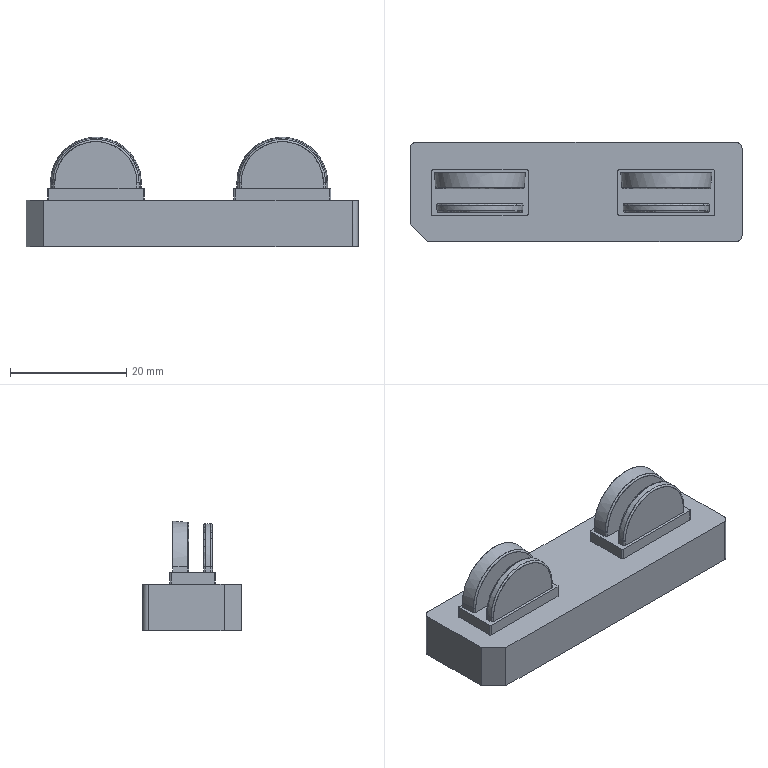NC program | PowerMill | posted by the shop | part box 57 x 17 x 18.807 mm
Lines 5595 to 7074 of 381081:
( TOOL ID   D4C_1_1 )
( TOOL DIA. 4. TIP RAD 0 LENGTH 66. )
( Z = -10.94 )
T2 M6
T28
G91 G28 Z0
G0 G90 G54
M08
S18000 M3
X0 Y0 M8
G43 Z9.797 H2
X-18.031 Y6.252
Z.788
G1 Z-.412 F3600
X-18.041 Y6.232 F6000
G3 X-17.952 Y5.967 I.177 J-.089
G1 X-16.594 Y5.288
X-14.886
X-14.398 Y5.259
X-13.942 Y5.125
X-13.421 Y4.791
X-13.258 Y4.637
X-12.93 Y4.148
X-12.77 Y3.66
X-12.737 Y3.172
X-12.828 Y2.684
X-12.975 Y2.196
X-13.19 Y1.708
X-13.925 Y.244
X-14.275 Y-.244
X-14.398 Y-.373
X-14.886 Y-.748
X-15.374 Y-1.024
X-15.862 Y-1.159
X-16.239 Y-1.22
X-16.747
X-17.326 Y-1.124
X-17.814 Y-.934
X-18.144 Y-.732
X-18.79 Y-.186
X-19.067 Y.244
X-19.81 Y1.708
X-20.026 Y2.196
X-20.172 Y2.684
X-20.26 Y3.172
X-20.23 Y3.66
X-20.07 Y4.148
X-19.766 Y4.607
X-19.278 Y5.011
X-19.057 Y5.125
X-18.79 Y5.218
X-18.302 Y5.288
X-16.594
X-18.019 Y6.246 Z-.612
X-18.029 Y6.226
G3 X-17.94 Y5.961 I.177 J-.089
G1 X-16.594 Y5.288
X-14.886
X-14.857 Y5.286
X-14.851
X-13.91
X-13.421 Y5.206
X-13.192 Y5.125
X-12.933 Y4.988
X-12.506 Y4.637
X-12.178 Y4.148
X-12.018 Y3.66
X-11.986 Y3.172
X-12.07 Y2.684
X-12.632 Y.732
X-12.74 Y.244
X-12.933 Y-.196
X-13.395 Y-.732
X-13.91 Y-1.072
X-14.072 Y-1.136
G3 X-14.179 Y-1.409 I.073 J-.186
G1 X-14.033 Y-1.708
X-13.947 Y-2.196
X-13.978 Y-2.684
X-14.121 Y-3.172
X-14.456 Y-3.66
X-15.374 Y-4.401
X-15.862 Y-4.645
X-16.35 Y-4.744
X-16.838 Y-4.721
X-17.145 Y-4.637
X-17.326 Y-4.571
X-17.814 Y-4.255
X-18.302 Y-3.885
X-18.545 Y-3.66
X-18.79 Y-3.324
X-18.869 Y-3.172
X-19.031 Y-2.684
X-19.054 Y-2.196
X-18.961 Y-1.708
X-18.814 Y-1.398
G3 X-18.911 Y-1.131 I-.181 J.086
G1 X-19.278 Y-.963
X-19.6 Y-.732
X-19.766 Y-.584
X-20.034 Y-.244
X-20.261 Y.244
X-20.368 Y.732
X-20.929 Y2.684
X-21.013 Y3.172
X-20.981 Y3.66
X-20.822 Y4.148
X-20.742 Y4.294
X-20.493 Y4.637
X-20.254 Y4.856
X-19.808 Y5.125
X-19.278 Y5.27
X-18.79 Y5.288
X-18.035
X-16.594
X-18.033 Y6.253 Z-.811
X-18.043 Y6.234
G3 X-17.955 Y5.968 I.177 J-.089
G1 X-16.594 Y5.288
X-14.886
X-14.866 Y5.287
X-13.421 Y5.286
X-12.933 Y5.205
X-12.706 Y5.125
X-12.445 Y4.987
X-12.019 Y4.637
X-11.691 Y4.148
X-11.53 Y3.66
X-11.5 Y3.172
X-12.119 Y.244
X-12.34 Y-.244
X-12.445 Y-.396
X-12.752 Y-.732
X-13.033 Y-.937
G3 X-13.075 Y-1.22 I.119 J-.162
G1 X-12.854 Y-1.708
X-12.762 Y-2.196
X-12.792 Y-2.684
X-13.017 Y-3.66
X-13.199 Y-4.148
X-13.421 Y-4.495
X-13.552 Y-4.637
X-13.91 Y-4.927
X-14.234 Y-5.125
X-14.398 Y-5.2
X-14.886 Y-5.341
X-15.374 Y-5.435
X-16.838 Y-5.478
X-17.814 Y-5.411
X-18.302 Y-5.294
X-18.765 Y-5.125
X-19.278 Y-4.789
X-19.449 Y-4.637
X-19.766 Y-4.216
X-19.976 Y-3.66
X-20.208 Y-2.684
X-20.238 Y-2.196
X-20.146 Y-1.708
X-19.925 Y-1.22
G3 X-19.968 Y-.955 I-.168 J.108
G1 X-20.248 Y-.732
X-20.658 Y-.244
X-20.742 Y-.098
X-20.882 Y.244
X-21.5 Y3.172
X-21.467 Y3.66
X-21.309 Y4.148
X-21.23 Y4.295
X-20.981 Y4.637
X-20.742 Y4.858
X-20.296 Y5.125
X-19.766 Y5.27
X-19.282 Y5.288
X-18.797
X-18.793
X-18.79
X-18.089
X-18.009
X-16.594
X-18.032 Y6.253 Z-1.01
X-18.042 Y6.233
G3 X-17.953 Y5.968 I.177 J-.089
G1 X-16.594 Y5.288
X-13.421
X-12.933 Y5.283
X-12.445 Y5.19
X-12.266 Y5.125
X-11.957 Y4.956
X-11.581 Y4.637
X-11.469 Y4.5
X-11.252 Y4.148
X-11.093 Y3.66
X-11.062 Y3.172
X-11.3 Y1.708
X-11.603 Y.244
X-11.825 Y-.244
X-12.216 Y-.732
X-12.392 Y-.87
G3 X-12.445 Y-1.123 I.123 J-.158
G1 X-12.177 Y-1.708
X-12.082 Y-2.196
X-12.114 Y-2.684
X-12.276 Y-3.66
X-12.445 Y-4.14
X-12.801 Y-4.637
X-12.933 Y-4.774
X-13.416 Y-5.125
X-13.91 Y-5.323
X-14.398 Y-5.437
X-14.886 Y-5.499
X-17.326 Y-5.524
X-18.302 Y-5.484
X-18.79 Y-5.404
X-19.278 Y-5.253
X-19.581 Y-5.125
X-19.766 Y-5.018
X-20.197 Y-4.637
X-20.55 Y-4.148
X-20.725 Y-3.66
X-20.889 Y-2.684
X-20.918 Y-2.196
X-20.826 Y-1.708
X-20.614 Y-1.22
X-20.57 Y-1.156
X-20.536 Y-1.086
G3 X-20.615 Y-.863 I-.194 J.057
G1 X-20.782 Y-.732
X-21.174 Y-.244
X-21.397 Y.244
X-21.718 Y1.798
X-21.939 Y3.172
X-21.907 Y3.66
X-21.747 Y4.148
X-21.419 Y4.637
X-21.23 Y4.816
X-20.742 Y5.12
X-20.254 Y5.263
X-19.766 Y5.288
X-16.594
X-18.033 Y6.253 Z-1.209
X-18.042 Y6.234
G3 X-17.954 Y5.968 I.177 J-.089
G1 X-16.594 Y5.288
X-12.933
X-12.445 Y5.273
X-11.957 Y5.15
X-11.469 Y4.875
X-11.208 Y4.637
X-10.981 Y4.333
X-10.879 Y4.148
X-10.72 Y3.66
X-10.689 Y3.172
X-11.168 Y.244
X-11.389 Y-.244
X-11.773 Y-.732
X-11.898 Y-.834
G3 X-11.938 Y-1.1 I.126 J-.155
G1 X-11.858 Y-1.22
X-11.656 Y-1.708
X-11.561 Y-2.196
X-11.591 Y-2.684
X-11.685 Y-3.172
X-11.742 Y-3.66
X-11.917 Y-4.148
X-12.247 Y-4.637
X-12.445 Y-4.839
X-12.86 Y-5.125
X-13.421 Y-5.364
X-13.91 Y-5.474
X-14.398 Y-5.513
X-16.945 Y-5.52
X-17.326 Y-5.524
X-17.39 Y-5.521
X-17.394
X-18.302 Y-5.524
X-18.79 Y-5.504
X-19.278 Y-5.435
X-19.766 Y-5.3
X-20.254 Y-5.06
X-20.752 Y-4.637
X-21.083 Y-4.148
X-21.23 Y-3.769
X-21.315 Y-3.172
X-21.409 Y-2.684
X-21.439 Y-2.196
X-21.347 Y-1.708
X-21.23 Y-1.389
X-21.144 Y-1.22
X-21.063 Y-1.101
G3 X-21.103 Y-.834 I-.166 J.112
G1 X-21.23 Y-.731
X-21.611 Y-.244
X-21.718 Y-.05
X-21.834 Y.244
X-22.311 Y3.172
X-22.28 Y3.66
X-22.12 Y4.148
X-21.792 Y4.637
X-21.23 Y5.066
X-20.742 Y5.241
X-20.254 Y5.288
X-16.594
X-18.029 Y6.251 Z-1.408
X-18.039 Y6.232
G3 X-17.95 Y5.966 I.177 J-.089
G1 X-16.594 Y5.288
X-12.933
X-12.929
X-12.445
X-11.957 Y5.25
X-11.551 Y5.125
X-10.981 Y4.755
X-10.866 Y4.637
X-10.537 Y4.148
X-10.377 Y3.66
X-10.346 Y3.172
X-10.406 Y2.684
X-10.792 Y.244
X-10.981 Y-.187
X-11.388 Y-.732
X-11.494 Y-.818
G3 X-11.532 Y-1.086 I.127 J-.155
G1 X-11.441 Y-1.22
X-11.234 Y-1.708
X-11.144 Y-2.196
X-11.172 Y-2.684
X-11.298 Y-3.66
X-11.473 Y-4.148
X-11.799 Y-4.637
X-11.957 Y-4.803
X-12.401 Y-5.125
X-12.933 Y-5.364
X-13.421 Y-5.481
X-13.91 Y-5.518
X-14.398 Y-5.524
X-18.79
X-19.278 Y-5.508
X-19.766 Y-5.445
X-20.254 Y-5.299
X-20.742 Y-5.037
X-21.201 Y-4.637
X-21.527 Y-4.148
X-21.7 Y-3.66
X-21.828 Y-2.684
X-21.857 Y-2.196
X-21.766 Y-1.708
X-21.557 Y-1.22
X-21.462 Y-1.081
G3 X-21.476 Y-.841 I-.159 J.111
G1 X-21.495 Y-.819
X-21.718 Y-.62
X-21.988 Y-.244
X-22.208 Y.244
X-22.526 Y2.196
X-22.654 Y3.172
X-22.624 Y3.66
X-22.463 Y4.148
X-22.206 Y4.554
X-21.718 Y4.985
X-21.45 Y5.125
X-21.23 Y5.204
X-20.742 Y5.286
X-20.271
X-20.254 Y5.288
X-16.594
X-18.031 Y6.253 Z-1.608
X-18.041 Y6.233
G3 X-17.953 Y5.967 I.177 J-.089
G1 X-16.594 Y5.288
X-12.933
X-12.929
X-12.445
X-12.416 Y5.286
X-12.409
X-11.957 Y5.285
X-11.469 Y5.201
X-11.255 Y5.125
X-10.981 Y4.978
X-10.57 Y4.637
X-10.242 Y4.148
X-10.082 Y3.66
X-10.051 Y3.172
X-10.387 Y.732
X-10.475 Y.244
X-10.691 Y-.244
X-10.981 Y-.648
X-11.15 Y-.797
G3 X-11.182 Y-1.061 I.132 J-.15
G1 X-11.071 Y-1.22
X-10.981 Y-1.4
X-10.872 Y-1.708
X-10.781 Y-2.196
X-10.811 Y-2.684
X-10.925 Y-3.66
X-10.981 Y-3.867
X-11.1 Y-4.148
X-11.406 Y-4.637
X-11.988 Y-5.125
X-12.445 Y-5.34
X-12.933 Y-5.469
X-13.421 Y-5.518
X-13.91 Y-5.524
X-19.278
X-19.766 Y-5.505
X-20.254 Y-5.427
X-20.742 Y-5.269
X-21.011 Y-5.125
X-21.23 Y-4.972
X-21.594 Y-4.637
X-21.718 Y-4.47
X-21.901 Y-4.148
X-22.076 Y-3.66
X-22.206 Y-2.559
X-22.219 Y-2.196
X-22.128 Y-1.708
X-21.929 Y-1.22
X-21.821 Y-1.066
G3 X-21.857 Y-.798 I-.164 J.114
G1 X-21.936 Y-.732
X-22.206 Y-.41
X-22.309 Y-.244
X-22.525 Y.244
X-22.613 Y.732
X-22.949 Y3.172
X-22.918 Y3.66
X-22.758 Y4.148
X-22.43 Y4.637
X-22.206 Y4.845
X-21.744 Y5.125
X-21.23 Y5.268
X-20.742 Y5.288
X-20.155
X-16.594
X-18.032 Y6.253 Z-1.807
X-18.042 Y6.234
G3 X-17.954 Y5.968 I.177 J-.089
G1 X-16.594 Y5.288
X-11.957
X-11.469 Y5.265
X-10.979 Y5.125
X-10.493 Y4.826
X-10.294 Y4.637
X-10.005 Y4.225
X-9.806 Y3.66
X-9.774 Y3.172
X-10.034 Y1.22
X-10.174 Y.244
X-10.381 Y-.244
X-10.493 Y-.425
X-10.753 Y-.732
X-10.809 Y-.778
X-10.857 Y-.832
G3 X-10.853 Y-1.055 I.168 J-.108
G1 X-10.738 Y-1.22
X-10.539 Y-1.708
X-10.45 Y-2.196
X-10.48 Y-2.684
X-10.587 Y-3.66
X-10.76 Y-4.148
X-11.073 Y-4.637
X-11.469 Y-4.994
X-11.653 Y-5.125
X-11.957 Y-5.283
X-12.445 Y-5.444
X-12.933 Y-5.513
X-13.421 Y-5.524
X-19.766
X-20.254 Y-5.494
X-20.742 Y-5.389
X-21.23 Y-5.192
X-21.718 Y-4.848
X-21.926 Y-4.637
X-22.206 Y-4.21
X-22.414 Y-3.66
X-22.488 Y-2.929
X-22.549 Y-2.196
X-22.461 Y-1.708
X-22.262 Y-1.22
X-22.146 Y-1.055
G3 X-22.192 Y-.778 I-.165 J.115
G1 X-22.247 Y-.732
X-22.62 Y-.244
X-22.826 Y.244
X-22.909 Y.732
X-23.226 Y3.172
X-23.195 Y3.66
X-23.035 Y4.148
X-22.706 Y4.637
X-22.206 Y5.033
X-22.021 Y5.125
X-21.718 Y5.226
X-21.23 Y5.288
X-16.594
X-18.029 Y6.251 Z-2.006
X-18.039 Y6.232
G3 X-17.95 Y5.966 I.177 J-.089
G1 X-16.594 Y5.288
X-11.957
X-11.946 Y5.287
X-11.469
X-10.981 Y5.215
X-10.724 Y5.125
X-10.493 Y5.006
X-10.039 Y4.637
X-9.711 Y4.148
X-9.551 Y3.66
X-9.52 Y3.172
X-9.815 Y.732
X-9.906 Y.244
X-10.121 Y-.244
X-10.493 Y-.731
X-10.562 Y-.793
X-10.606 Y-.874
X-10.61 Y-.963
X-10.574 Y-1.044
X-10.493 Y-1.155
X-10.257 Y-1.708
X-10.172 Y-2.196
X-10.301 Y-3.66
X-10.47 Y-4.148
X-10.773 Y-4.637
X-10.981 Y-4.847
X-11.337 Y-5.125
X-11.469 Y-5.201
X-11.957 Y-5.401
X-12.445 Y-5.497
X-12.933 Y-5.524
X-13.417
X-13.419
X-13.421
X-19.766
X-19.786 Y-5.523
X-20.254
X-20.742 Y-5.474
X-21.23 Y-5.334
X-21.662 Y-5.125
X-22.206 Y-4.659
X-22.53 Y-4.148
X-22.699 Y-3.66
X-22.828 Y-2.196
X-22.694 Y-1.55
X-22.545 Y-1.22
X-22.421 Y-1.044
G3 X-22.439 Y-.791 I-.163 J.115
G1 X-22.694 Y-.523
X-22.879 Y-.244
X-23.094 Y.244
X-23.183 Y.711
X-23.48 Y3.172
X-23.449 Y3.66
X-23.289 Y4.148
X-23.183 Y4.343
X-22.961 Y4.637
X-22.694 Y4.879
X-22.274 Y5.125
X-21.718 Y5.273
X-21.23 Y5.288
X-20.394
X-16.594
X-18.029 Y6.251 Z-2.205
X-18.038 Y6.232
G3 X-17.95 Y5.966 I.177 J-.089
G1 X-16.594 Y5.288
X-11.469
X-10.981 Y5.262
X-10.503 Y5.125
X-10.005 Y4.815
X-9.818 Y4.637
X-9.517 Y4.202
X-9.33 Y3.66
X-9.299 Y3.172
X-9.575 Y.732
X-9.659 Y.244
X-9.863 Y-.244
X-10.005 Y-.468
X-10.235 Y-.732
X-10.299 Y-.791
X-10.34 Y-.868
X-10.344 Y-.955
X-10.311 Y-1.036
X-10.181 Y-1.22
X-10.005 Y-1.632
X-9.898 Y-2.196
X-9.919 Y-2.684
X-10.005 Y-3.554
X-10.196 Y-4.148
X-10.499 Y-4.637
X-11.063 Y-5.125
X-11.469 Y-5.323
X-11.957 Y-5.47
X-12.445 Y-5.523
X-12.915
X-12.933 Y-5.524
X-13.417
X-13.419
X-13.421
X-19.766
X-19.769
X-19.771
X-20.257
X-20.742 Y-5.509
X-21.23 Y-5.428
X-21.718 Y-5.246
X-21.936 Y-5.125
X-22.206 Y-4.92
X-22.501 Y-4.637
X-22.694 Y-4.363
X-22.804 Y-4.148
X-22.975 Y-3.66
X-23.036 Y-3.172
X-23.102 Y-2.196
X-23.017 Y-1.708
X-22.819 Y-1.22
X-22.689 Y-1.037
G3 X-22.721 Y-.77 I-.163 J.115
G1 X-22.765 Y-.732
X-23.138 Y-.244
X-23.341 Y.244
X-23.425 Y.732
X-23.7 Y3.172
X-23.671 Y3.655
X-23.51 Y4.148
X-23.182 Y4.637
X-22.694 Y5.025
X-22.495 Y5.125
X-22.206 Y5.224
X-21.718 Y5.288
X-16.594
X-18.033 Y6.253 Z-2.405
X-18.043 Y6.234
G3 X-17.954 Y5.968 I.177 J-.089
G1 X-16.594 Y5.288
X-11.469
X-11.421 Y5.285
X-11.416
X-10.981
X-10.493 Y5.2
X-10.282 Y5.125
X-10.005 Y4.976
X-9.597 Y4.637
X-9.269 Y4.148
X-9.109 Y3.66
X-9.078 Y3.172
X-9.353 Y.732
X-9.437 Y.244
X-9.645 Y-.244
X-10.018 Y-.732
X-10.092 Y-.813
X-10.12 Y-.92
X-10.109 Y-.977
X-10.083 Y-1.029
X-9.947 Y-1.22
X-9.75 Y-1.708
X-9.662 Y-2.196
X-9.781 Y-3.66
X-9.951 Y-4.148
X-10.254 Y-4.637
X-10.493 Y-4.877
X-10.807 Y-5.125
X-10.981 Y-5.224
X-11.469 Y-5.421
X-11.957 Y-5.506
X-12.445 Y-5.524
X-20.742
X-21.23 Y-5.485
X-21.718 Y-5.356
X-22.194 Y-5.125
X-22.694 Y-4.694
X-23.049 Y-4.148
X-23.219 Y-3.66
X-23.337 Y-2.196
X-23.25 Y-1.708
X-23.183 Y-1.499
X-23.053 Y-1.22
X-22.912 Y-1.021
G3 X-22.932 Y-.765 I-.163 J.116
G1 X-23.183 Y-.509
X-23.355 Y-.244
X-23.563 Y.244
X-23.647 Y.732
X-23.921 Y3.172
X-23.891 Y3.66
X-23.73 Y4.148
X-23.403 Y4.637
X-23.183 Y4.843
X-22.716 Y5.125
X-22.206 Y5.268
X-21.723 Y5.288
X-21.238
X-16.594
X-18.021 Y6.247 Z-2.604
X-18.031 Y6.228
G3 X-17.942 Y5.962 I.177 J-.089
G1 X-16.594 Y5.288
X-11.507
X-10.981
X-10.493 Y5.251
X-10.085 Y5.125
X-9.517 Y4.754
X-9.4 Y4.637
X-9.072 Y4.148
X-8.912 Y3.66
X-8.88 Y3.172
X-9.138 Y.732
X-9.226 Y.244
X-9.428 Y-.244
X-9.517 Y-.392
X-9.801 Y-.732
X-9.871 Y-.812
X-9.896 Y-.915
X-9.886 Y-.972
X-9.859 Y-1.023
X-9.719 Y-1.22
X-9.522 Y-1.708
X-9.438 Y-2.196
X-9.468 Y-2.684
X-9.557 Y-3.66
X-9.723 Y-4.148
X-10.005 Y-4.609
X-10.579 Y-5.125
X-10.981 Y-5.325
X-11.469 Y-5.474
X-11.957 Y-5.524
X-20.742
X-21.23 Y-5.514
X-21.718 Y-5.432
X-22.206 Y-5.243
X-22.422 Y-5.125
X-22.694 Y-4.914
X-22.973 Y-4.637
X-23.183 Y-4.335
X-23.276 Y-4.148
X-23.443 Y-3.66
X-23.561 Y-2.196
X-23.478 Y-1.708
X-23.281 Y-1.22
X-23.141 Y-1.023
G3 X-23.179 Y-.75 I-.164 J.116
G1 X-23.199 Y-.732
X-23.573 Y-.244
X-23.774 Y.244
X-23.862 Y.732
X-24.12 Y3.172
X-24.088 Y3.66
X-23.928 Y4.148
X-23.6 Y4.637
X-23.183 Y4.984
X-22.915 Y5.125
X-22.694 Y5.203
X-22.206 Y5.286
X-21.775
X-21.718 Y5.288
X-21.238
X-16.594
X-18.03 Y6.252 Z-2.803
X-18.04 Y6.232
G3 X-17.951 Y5.967 I.177 J-.089
G1 X-16.594 Y5.288
X-10.981
X-10.493 Y5.277
X-10.005 Y5.164
X-9.517 Y4.902
X-9.221 Y4.637
X-9.029 Y4.391
X-8.892 Y4.148
X-8.732 Y3.66
X-8.701 Y3.172
X-8.951 Y.732
X-9.035 Y.244
X-9.237 Y-.244
X-9.517 Y-.636
X-9.638 Y-.756
G3 X-9.662 Y-1.012 I.141 J-.142
G1 X-9.517 Y-1.22
X-9.32 Y-1.708
X-9.232 Y-2.196
X-9.252 Y-2.684
X-9.346 Y-3.66
X-9.512 Y-4.148
X-9.816 Y-4.637
X-10.005 Y-4.836
X-10.358 Y-5.125
X-10.493 Y-5.203
X-10.981 Y-5.411
X-11.469 Y-5.504
X-11.957 Y-5.524
X-21.23
X-21.718 Y-5.48
X-22.206 Y-5.342
X-22.64 Y-5.125
X-23.184 Y-4.637
X-23.488 Y-4.148
X-23.654 Y-3.66
X-23.712 Y-3.172
X-23.768 Y-2.196
X-23.68 Y-1.708
X-23.483 Y-1.22
X-23.34 Y-1.015
G3 X-23.347 Y-.779 I-.158 J.113
G1 X-23.365 Y-.757
X-23.39 Y-.732
X-23.671 Y-.396
X-23.763 Y-.244
X-23.965 Y.244
X-24.049 Y.732
X-24.299 Y3.172
X-24.268 Y3.66
X-24.108 Y4.148
X-23.78 Y4.637
X-23.671 Y4.747
X-23.183 Y5.083
X-22.694 Y5.249
X-22.206 Y5.288
X-21.713
X-16.594
X-18.027 Y6.251 Z-3.003
X-18.037 Y6.231
G3 X-17.949 Y5.965 I.177 J-.089
G1 X-16.594 Y5.288
X-10.981
X-10.97
X-10.493
X-10.005 Y5.221
X-9.726 Y5.125
X-9.517 Y5.019
X-9.042 Y4.637
X-8.712 Y4.148
X-8.553 Y3.66
X-8.521 Y3.172
X-8.768 Y.732
X-8.851 Y.244
X-9.029 Y-.195
X-9.428 Y-.732
G3 X-9.473 Y-1.01 I.123 J-.163
G1 X-9.326 Y-1.22
X-9.129 Y-1.708
X-9.043 Y-2.196
X-9.153 Y-3.66
X-9.322 Y-4.148
X-9.517 Y-4.495
X-9.626 Y-4.637
X-10.005 Y-5.008
X-10.168 Y-5.125
X-10.493 Y-5.295
X-10.981 Y-5.461
X-11.469 Y-5.523
X-11.933
X-11.937
X-11.957 Y-5.524
X-20.738
X-21.228
X-21.718 Y-5.508
X-22.206 Y-5.413
X-22.694 Y-5.204
X-22.831 Y-5.125
X-23.183 Y-4.839
X-23.374 Y-4.637
X-23.671 Y-4.165
X-23.847 Y-3.66
X-23.957 Y-2.196
X-23.871 Y-1.708
X-23.671 Y-1.215
X-23.526 Y-1.009
G3 X-23.548 Y-.752 I-.164 J.115
G1 X-23.671 Y-.63
X-23.945 Y-.244
X-24.149 Y.244
X-24.233 Y.732
X-24.479 Y3.172
X-24.447 Y3.66
X-24.288 Y4.148
X-24.159 Y4.376
X-23.959 Y4.637
X-23.671 Y4.895
X-23.274 Y5.125
X-22.694 Y5.275
X-22.206 Y5.288
X-20.301
X-16.594
X-18.032 Y6.253 Z-3.202
X-18.041 Y6.233
G3 X-17.953 Y5.967 I.177 J-.089
G1 X-16.594 Y5.288
X-12.922
X-10.493
X-10.005 Y5.257
X-9.56 Y5.125
X-9.029 Y4.788
X-8.875 Y4.637
X-8.546 Y4.148
X-8.387 Y3.66
X-8.355 Y3.172
X-8.603 Y.732
X-8.687 Y.244
X-8.882 Y-.244
X-9.029 Y-.473
X-9.28 Y-.749
G3 X-9.298 Y-.997 I.148 J-.135
G1 X-9.145 Y-1.22
X-9.029 Y-1.461
X-8.948 Y-1.708
X-8.87 Y-2.196
X-8.976 Y-3.66
X-9.134 Y-4.148
X-9.437 Y-4.637
X-9.978 Y-5.125
X-10.493 Y-5.376
X-10.981 Y-5.492
X-11.469 Y-5.524
X-13.289
X-20.738
X-21.23
X-21.252 Y-5.523
X-21.718
X-22.206 Y-5.462
X-22.694 Y-5.296
X-23.022 Y-5.125
X-23.183 Y-5.01
X-23.563 Y-4.637
X-23.671 Y-4.496
X-23.866 Y-4.148
X-24.024 Y-3.66
X-24.131 Y-2.196
X-24.052 Y-1.708
X-23.855 Y-1.22
X-23.707 Y-1.004
G3 X-23.741 Y-.739 I-.166 J.113
G1 X-23.748 Y-.732
X-24.117 Y-.244
X-24.313 Y.244
X-24.397 Y.732
X-24.645 Y3.172
X-24.613 Y3.66
X-24.454 Y4.148
X-24.159 Y4.598
X-23.671 Y5.007
X-23.438 Y5.125
X-23.183 Y5.215
X-22.694 Y5.287
X-22.22
X-22.206 Y5.288
X-20.301
X-16.594
X-18.032 Y6.253 Z-3.401
X-18.042 Y6.234
G3 X-17.954 Y5.968 I.177 J-.089
G1 X-16.594 Y5.288
X-10.493
X-10.005 Y5.276
X-9.517 Y5.163
X-9.029 Y4.899
X-8.735 Y4.637
X-8.541 Y4.387
X-8.406 Y4.148
X-8.247 Y3.66
X-8.215 Y3.172
X-8.447 Y.732
X-8.533 Y.244
X-8.73 Y-.244
X-9.029 Y-.657
X-9.093 Y-.719
X-9.147 Y-.789
G3 X-9.135 Y-.999 I.176 J-.095
G1 X-9.029 Y-1.149
X-8.789 Y-1.708
X-8.703 Y-2.196
X-8.721 Y-2.684
X-8.813 Y-3.66
X-8.975 Y-4.148
X-9.278 Y-4.637
X-9.517 Y-4.892
X-9.814 Y-5.125
X-10.005 Y-5.231
X-10.493 Y-5.432
X-10.981 Y-5.515
X-11.469 Y-5.524
X-21.718
X-22.206 Y-5.491
X-22.694 Y-5.371
X-23.183 Y-5.127
X-23.671 Y-4.693
X-24.025 Y-4.148
X-24.159 Y-3.771
X-24.243 Y-3.172
X-24.296 Y-2.196
X-24.211 Y-1.708
X-24.014 Y-1.22
X-23.858 Y-.993
G3 X-23.882 Y-.737 I-.166 J.113
G1 X-24.159 Y-.426
X-24.271 Y-.244
X-24.468 Y.244
X-24.553 Y.732
X-24.785 Y3.172
X-24.753 Y3.66
X-24.593 Y4.148
X-24.265 Y4.637
X-24.159 Y4.743
X-23.671 Y5.082
X-23.183 Y5.248
X-22.694 Y5.288
X-16.594
X-18.022 Y6.248 Z-3.6
X-18.032 Y6.228
G3 X-17.943 Y5.963 I.177 J-.089
G1 X-16.594 Y5.288
X-10.493
X-10.451 Y5.287
X-10.449
X-10.005
X-9.517 Y5.211
X-9.275 Y5.125
X-9.029 Y4.997
X-8.589 Y4.637
X-8.261 Y4.148
X-8.101 Y3.66
X-8.07 Y3.172
X-8.297 Y.732
X-8.381 Y.244
X-8.541 Y-.176
X-8.946 Y-.732
G3 X-8.98 Y-.997 I.132 J-.152
G1 X-8.827 Y-1.22
X-8.63 Y-1.708
X-8.552 Y-2.196
X-8.659 Y-3.66
X-8.817 Y-4.148
X-9.029 Y-4.52
X-9.119 Y-4.637
X-9.517 Y-5.027
X-9.655 Y-5.125
X-10.005 Y-5.311
X-10.493 Y-5.469
X-10.981 Y-5.524
X-21.718
X-22.206 Y-5.513
X-22.694 Y-5.425
X-23.183 Y-5.217
X-23.345 Y-5.125
X-23.671 Y-4.864
X-23.88 Y-4.637
X-24.159 Y-4.203
X-24.342 Y-3.66
X-24.449 Y-2.196
X-24.37 Y-1.708
X-24.159 Y-1.198
X-24.019 Y-.995
G3 X-24.04 Y-.743 I-.165 J.113
G1 X-24.159 Y-.621
X-24.424 Y-.244
X-24.619 Y.244
X-24.702 Y.732
X-24.93 Y3.172
X-24.899 Y3.66
X-24.738 Y4.148
X-24.647 Y4.318
X-24.41 Y4.637
X-24.159 Y4.867
X-23.725 Y5.125
X-23.183 Y5.272
X-22.694 Y5.288
X-22.062
X-16.594
X-18.029 Y6.252 Z-3.799
X-18.039 Y6.232
G3 X-17.95 Y5.966 I.177 J-.089
G1 X-16.594 Y5.288
X-10.005
X-9.517 Y5.244
X-9.029 Y5.074
X-8.541 Y4.727
X-8.453 Y4.637
X-8.124 Y4.148
X-7.965 Y3.66
X-7.933 Y3.172
X-8.164 Y.732
X-8.247 Y.244
X-8.441 Y-.244
X-8.541 Y-.407
X-8.831 Y-.742
G3 X-8.846 Y-.985 I.151 J-.131
G1 X-8.687 Y-1.22
X-8.49 Y-1.708
X-8.412 Y-2.196
X-8.516 Y-3.66
X-8.671 Y-4.148
X-8.974 Y-4.637
X-9.504 Y-5.125
X-10.005 Y-5.377
X-10.493 Y-5.494
X-10.981 Y-5.524
X-11.739
X-21.718
X-21.779 Y-5.523
X-22.206
X-22.694 Y-5.462
X-23.183 Y-5.297
X-23.496 Y-5.125
X-23.671 Y-4.998
X-24.026 Y-4.637
X-24.159 Y-4.459
X-24.329 Y-4.148
X-24.485 Y-3.66
X-24.587 Y-2.196
X-24.51 Y-1.708
X-24.313 Y-1.22
X-24.161 Y-.994
G3 X-24.177 Y-.752 I-.162 J.111
G1 X-24.185 Y-.742
X-24.194 Y-.732
X-24.559 Y-.244
X-24.753 Y.244
X-24.836 Y.732
X-25.067 Y3.172
X-25.035 Y3.66
X-24.875 Y4.148
X-24.647 Y4.518
X-24.547 Y4.637
X-24.159 Y4.966
X-23.861 Y5.125
X-23.671 Y5.196
X-23.183 Y5.284
X-22.694 Y5.288
X-16.594
X-18.032 Y6.253 Z-3.999
X-18.042 Y6.233
G3 X-17.953 Y5.968 I.177 J-.089
G1 X-16.594 Y5.288
X-10.005
X-9.517 Y5.267
X-9.016 Y5.125
X-8.541 Y4.835
X-8.33 Y4.637
X-8.002 Y4.148
X-7.842 Y3.66
X-7.811 Y3.172
X-8.03 Y.732
X-8.116 Y.244
X-8.315 Y-.244
X-8.541 Y-.575
X-8.694 Y-.739
G3 X-8.715 Y-.986 I.146 J-.136
G1 X-8.541 Y-1.248
X-8.358 Y-1.708
X-8.281 Y-2.196
X-8.299 Y-2.684
X-8.384 Y-3.66
X-8.541 Y-4.151
X-8.843 Y-4.637
X-9.029 Y-4.845
X-9.373 Y-5.125
X-10.005 Y-5.42
X-10.493 Y-5.513
X-10.981 Y-5.524
X-22.206
X-22.694 Y-5.486
X-23.183 Y-5.355
X-23.627 Y-5.125
X-24.159 Y-4.634
X-24.461 Y-4.148
X-24.616 Y-3.66
X-24.647 Y-3.48
X-24.719 Y-2.196
X-24.641 Y-1.708
X-24.445 Y-1.22
X-24.29 Y-.992
X-24.257 Y-.902
X-24.271 Y-.808
X-24.291 Y-.767
X-24.321 Y-.732
X-24.647 Y-.311
X-24.884 Y.244
X-24.97 Y.732
X-25.189 Y3.172
X-25.157 Y3.66
X-24.998 Y4.148
X-24.669 Y4.637
X-24.159 Y5.038
X-23.983 Y5.125
X-23.671 Y5.23
X-23.183 Y5.288
X-16.594
X-18.027 Y6.25 Z-4.198
X-18.037 Y6.231
G3 X-17.948 Y5.965 I.177 J-.089
G1 X-16.594 Y5.288
X-10.005
X-9.517 Y5.278
X-9.029 Y5.172
X-8.541 Y4.918
X-8.221 Y4.637
X-8.053 Y4.425
X-7.892 Y4.148
X-7.733 Y3.66
X-7.701 Y3.172
X-7.911 Y.732
X-7.995 Y.244
X-8.188 Y-.244
X-8.552 Y-.732
X-8.558 Y-.739
X-8.563 Y-.745
G3 X-8.58 Y-.989 I.145 J-.133
G1 X-8.424 Y-1.22
X-8.227 Y-1.708
X-8.15 Y-2.196
X-8.168 Y-2.684
X-8.252 Y-3.66
X-8.408 Y-4.148
X-8.541 Y-4.401
X-8.712 Y-4.637
X-9.029 Y-4.966
X-9.241 Y-5.125
X-9.517 Y-5.278
X-10.005 Y-5.454
X-10.493 Y-5.523
X-10.924
X-10.981 Y-5.524
X-21.752
X-22.224
X-22.694 Y-5.506
X-23.183 Y-5.403
X-23.671 Y-5.177
X-24.159 Y-4.786
X-24.289 Y-4.637
X-24.592 Y-4.148
X-24.749 Y-3.66
X-24.801 Y-3.172
X-24.85 Y-2.196
X-24.772 Y-1.708
X-24.647 Y-1.357
X-24.409 Y-.981
G3 X-24.429 Y-.74 I-.169 J.107
G1 X-24.647 Y-.498
X-24.812 Y-.244
X-25.005 Y.244
X-25.088 Y.732
X-25.299 Y3.172
X-25.267 Y3.66
X-25.135 Y4.089
X-24.779 Y4.637
X-24.647 Y4.768
X-24.159 Y5.095
X-23.671 Y5.254
X-23.183 Y5.288
X-16.594
X-18.031 Y6.253 Z-4.397
X-18.041 Y6.233
G3 X-17.952 Y5.967 I.177 J-.089
G1 X-16.594 Y5.288
X-10.005
X-9.958 Y5.287
X-9.956
X-9.517
X-9.029 Y5.21
X-8.789 Y5.125
X-8.541 Y4.996
X-8.106 Y4.637
X-7.776 Y4.148
X-7.616 Y3.66
X-7.585 Y3.172
X-7.801 Y.732
X-7.885 Y.244
X-8.053 Y-.188
X-8.442 Y-.732
G3 X-8.47 Y-.987 I.139 J-.144
G1 X-8.314 Y-1.22
X-8.118 Y-1.708
X-8.034 Y-2.196
X-8.135 Y-3.66
X-8.294 Y-4.148
X-8.541 Y-4.565
X-9.029 Y-5.059
X-9.124 Y-5.125
X-9.517 Y-5.337
X-10.005 Y-5.479
X-10.493 Y-5.524
X-22.206
X-22.694 Y-5.518
X-23.183 Y-5.44
X-23.671 Y-5.244
X-23.876 Y-5.125
X-24.159 Y-4.905
X-24.402 Y-4.637
X-24.647 Y-4.272
X-24.865 Y-3.66
X-24.965 Y-2.196
X-24.883 Y-1.708
X-24.686 Y-1.22
X-24.53 Y-.987
G3 X-24.558 Y-.732 I-.167 J.111
G1 X-24.918 Y-.244
X-25.115 Y.244
X-25.199 Y.732
X-25.415 Y3.172
X-25.384 Y3.66
X-25.224 Y4.148
X-25.135 Y4.315
X-24.896 Y4.637
X-24.647 Y4.866
X-24.211 Y5.125
X-23.671 Y5.27
X-23.183 Y5.288
X-22.447
X-16.594
X-18.032 Y6.253 Z-4.596
X-18.042 Y6.234
G3 X-17.954 Y5.968 I.177 J-.089
G1 X-16.594 Y5.288
X-9.517
X-9.029 Y5.235
X-8.541 Y5.051
X-8.053 Y4.682
X-7.681 Y4.148
X-7.521 Y3.66
X-7.49 Y3.172
X-7.698 Y.732
X-7.782 Y.244
X-7.978 Y-.244
X-8.053 Y-.369
X-8.359 Y-.734
G3 X-8.372 Y-.974 I.153 J-.128
G1 X-8.207 Y-1.22
X-8.053 Y-1.565
X-7.93 Y-2.196
X-8.029 Y-3.66
X-8.187 Y-4.148
X-8.491 Y-4.637
X-9.017 Y-5.125
X-9.517 Y-5.38
X-10.005 Y-5.498
X-10.493 Y-5.524
X-18.513
X-22.206
X-22.209
X-22.694
X-23.183 Y-5.464
X-23.671 Y-5.3
X-23.983 Y-5.125
X-24.159 Y-4.998
X-24.509 Y-4.637
X-24.647 Y-4.453
X-24.812 Y-4.148
X-24.972 Y-3.66
X-25.071 Y-2.196
X-24.99 Y-1.708
X-24.793 Y-1.22
X-24.636 Y-.985
G3 X-24.655 Y-.74 I-.164 J.111
G1 X-24.658 Y-.736
X-24.661 Y-.732
X-25.022 Y-.244
X-25.218 Y.244
X-25.302 Y.732
X-25.51 Y3.172
X-25.478 Y3.66
X-25.319 Y4.148
X-25.135 Y4.458
X-24.99 Y4.637
X-24.647 Y4.936
X-24.305 Y5.125
X-24.159 Y5.181
X-23.671 Y5.281
X-23.183 Y5.288
X-16.594
X-18.033 Y6.253 Z-4.796
X-18.042 Y6.234
G3 X-17.954 Y5.968 I.177 J-.089
G1 X-16.594 Y5.288
X-10.391
X-9.517
X-9.029 Y5.255
X-8.599 Y5.125
X-8.053 Y4.775
X-7.913 Y4.637
X-7.584 Y4.148
X-7.425 Y3.66
X-7.393 Y3.172
X-7.599 Y.732
X-7.684 Y.244
X-7.875 Y-.244
X-8.053 Y-.517
X-8.245 Y-.732
G3 X-8.263 Y-.976 I.149 J-.134
G1 X-8.1 Y-1.22
X-7.904 Y-1.708
X-7.827 Y-2.196
X-7.926 Y-3.66
X-8.053 Y-4.083
X-8.384 Y-4.637
X-8.541 Y-4.819
X-8.91 Y-5.125
X-9.517 Y-5.415
X-10.005 Y-5.512
X-10.493 Y-5.524
X-22.694
X-23.183 Y-5.483
X-23.671 Y-5.347
X-24.09 Y-5.125
X-24.616 Y-4.637
X-24.919 Y-4.148
X-25.074 Y-3.66
X-25.173 Y-2.196
X-25.097 Y-1.708
X-24.899 Y-1.22
X-24.741 Y-.983
G3 X-24.748 Y-.754 I-.16 J.11
G1 X-24.764 Y-.732
X-25.135 Y-.227
X-25.317 Y.244
X-25.401 Y.732
X-25.607 Y3.172
X-25.575 Y3.66
X-25.415 Y4.148
X-25.135 Y4.582
X-24.647 Y4.998
X-24.402 Y5.125
X-24.159 Y5.211
X-23.671 Y5.287
X-23.238
X-23.183 Y5.288
X-16.594
X-18.02 Y6.247 Z-4.995
X-18.029 Y6.227
G3 X-17.941 Y5.962 I.177 J-.089
G1 X-16.594 Y5.288
X-9.517
X-9.029 Y5.268
X-8.541 Y5.136
X-8.053 Y4.846
X-7.829 Y4.637
X-7.565 Y4.271
X-7.5 Y4.148
X-7.341 Y3.66
X-7.31 Y3.172
X-7.516 Y.732
X-7.565 Y.375
X-7.791 Y-.244
X-8.053 Y-.619
X-8.156 Y-.731
G3 X-8.175 Y-.976 I.147 J-.135
G1 X-8.014 Y-1.22
X-7.817 Y-1.708
X-7.739 Y-2.196
X-7.755 Y-2.684
X-7.837 Y-3.66
X-7.991 Y-4.148
X-8.293 Y-4.637
X-8.541 Y-4.91
X-8.817 Y-5.125
X-9.029 Y-5.25
X-9.517 Y-5.443
X-10.005 Y-5.518
X-10.493 Y-5.524
X-22.694
X-23.183 Y-5.5
X-23.671 Y-5.386
X-24.159 Y-5.14
X-24.647 Y-4.712
X-25.009 Y-4.148
X-25.135 Y-3.775
X-25.216 Y-3.172
X-25.261 Y-2.196
X-25.183 Y-1.708
X-24.986 Y-1.22
X-24.828 Y-.982
G3 X-24.836 Y-.754 I-.161 J.109
G1 X-24.852 Y-.732
X-25.209 Y-.244
X-25.401 Y.244
X-25.484 Y.732
X-25.691 Y3.172
X-25.659 Y3.66
X-25.5 Y4.148
X-25.171 Y4.637
X-24.647 Y5.046
X-24.486 Y5.125
X-24.159 Y5.233
X-23.671 Y5.288
X-16.594
X-18.024 Y6.249 Z-5.194